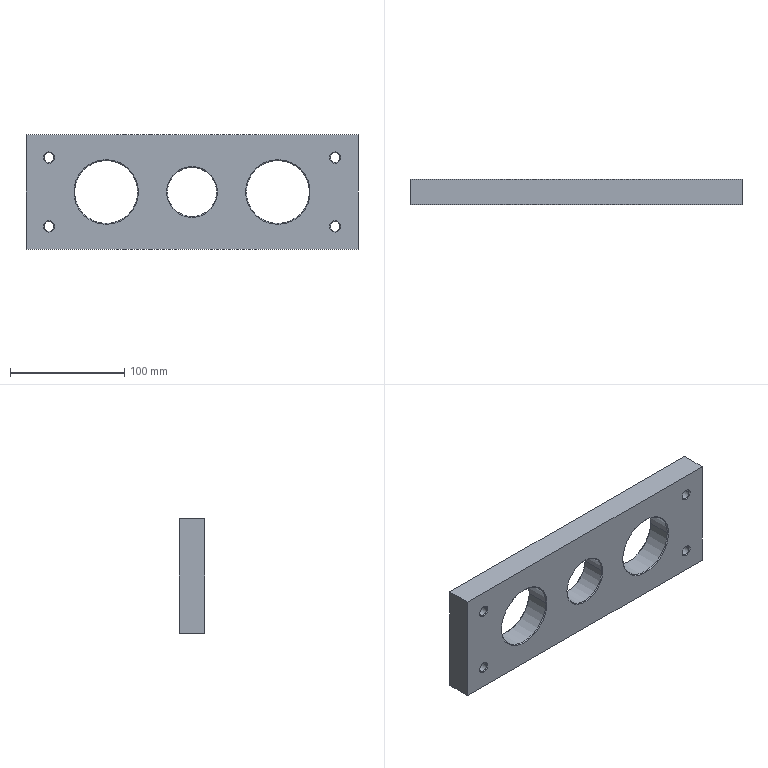Part | STEP file | BCC3 H13_1 | 1 solid | 48 faces | box 290 x 22 x 100 mm | volume 496185 mm3 | cone 28 | cylinder 14 | plane 6 | commonest cylinder face diameters 8.5 x8 55 x4 43 x2